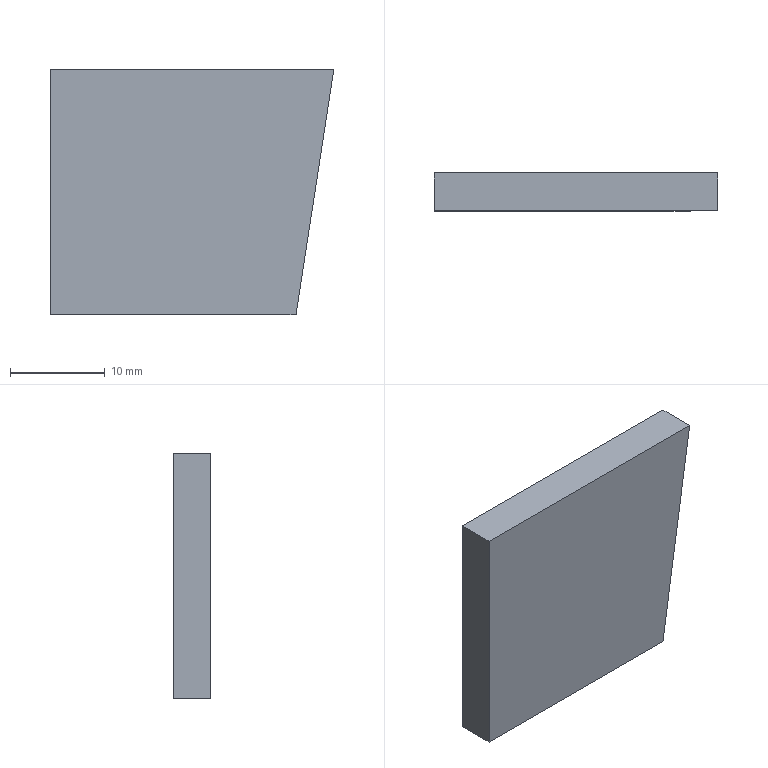Part | SolidWorks | features Extrusion 1 | 1 solid | 6 faces | box 30 x 4 x 26 mm | volume 2912 mm3 | plane 6
STEP:
#1=CARTESIAN_POINT('',(0.,0.,0.));
#2=VERTEX_POINT('',#1);
#3=CARTESIAN_POINT('',(30.,0.,0.));
#4=VERTEX_POINT('',#3);
#5=CARTESIAN_POINT('',(30.,0.,0.));
#6=DIRECTION('',(1.,0.,0.));
#7=VECTOR('',#6,1000.);
#8=LINE('',#5,#7);
#9=EDGE_CURVE('',#2,#4,#8,.T.);
#10=ORIENTED_EDGE('',*,*,#9,.T.);
#11=CARTESIAN_POINT('',(30.,4.,0.));
#12=VERTEX_POINT('',#11);
#13=CARTESIAN_POINT('',(30.,4.,0.));
#14=DIRECTION('',(0.,-1.,0.));
#15=VECTOR('',#14,1000.);
#16=LINE('',#13,#15);
#17=EDGE_CURVE('',#12,#4,#16,.T.);
#18=ORIENTED_EDGE('',*,*,#17,.F.);
#19=CARTESIAN_POINT('',(0.,4.,0.));
#20=VERTEX_POINT('',#19);
#21=CARTESIAN_POINT('',(30.,4.,0.));
#22=DIRECTION('',(1.,0.,0.));
#23=VECTOR('',#22,1000.);
#24=LINE('',#21,#23);
#25=EDGE_CURVE('',#20,#12,#24,.T.);
#26=ORIENTED_EDGE('',*,*,#25,.F.);
#27=CARTESIAN_POINT('',(0.,4.,0.));
#28=DIRECTION('',(0.,-1.,0.));
#29=VECTOR('',#28,1000.);
#30=LINE('',#27,#29);
#31=EDGE_CURVE('',#20,#2,#30,.T.);
#32=ORIENTED_EDGE('',*,*,#31,.T.);
#33=EDGE_LOOP('',(#10,#18,#26,#32));
#34=FACE_OUTER_BOUND('',#33,.T.);
#35=CARTESIAN_POINT('',(30.,4.,0.));
#36=DIRECTION('',(0.,0.,-1.));
#37=DIRECTION('',(-1.,0.,0.));
#38=AXIS2_PLACEMENT_3D('',#35,#36,#37);
#39=PLANE('',#38);
#40=ADVANCED_FACE('',(#34),#39,.F.);
#41=CARTESIAN_POINT('',(26.,0.,-26.));
#42=VERTEX_POINT('',#41);
#43=CARTESIAN_POINT('',(26.,0.,-26.));
#44=DIRECTION('',(-0.1521,0.,-0.9884));
#45=VECTOR('',#44,1000.);
#46=LINE('',#43,#45);
#47=EDGE_CURVE('',#4,#42,#46,.T.);
#48=ORIENTED_EDGE('',*,*,#47,.T.);
#49=CARTESIAN_POINT('',(26.,4.,-26.));
#50=VERTEX_POINT('',#49);
#51=CARTESIAN_POINT('',(26.,4.,-26.));
#52=DIRECTION('',(0.,-1.,0.));
#53=VECTOR('',#52,1000.);
#54=LINE('',#51,#53);
#55=EDGE_CURVE('',#50,#42,#54,.T.);
#56=ORIENTED_EDGE('',*,*,#55,.F.);
#57=CARTESIAN_POINT('',(26.,4.,-26.));
#58=DIRECTION('',(-0.1521,0.,-0.9884));
#59=VECTOR('',#58,1000.);
#60=LINE('',#57,#59);
#61=EDGE_CURVE('',#12,#50,#60,.T.);
#62=ORIENTED_EDGE('',*,*,#61,.F.);
#63=ORIENTED_EDGE('',*,*,#17,.T.);
#64=EDGE_LOOP('',(#48,#56,#62,#63));
#65=FACE_OUTER_BOUND('',#64,.T.);
#66=CARTESIAN_POINT('',(26.,4.,-26.));
#67=DIRECTION('',(-0.9884,0.,0.1521));
#68=DIRECTION('',(0.1521,0.,0.9884));
#69=AXIS2_PLACEMENT_3D('',#66,#67,#68);
#70=PLANE('',#69);
#71=ADVANCED_FACE('',(#65),#70,.F.);
#72=CARTESIAN_POINT('',(0.,0.,-26.));
#73=VERTEX_POINT('',#72);
#74=CARTESIAN_POINT('',(0.,0.,-26.));
#75=DIRECTION('',(-1.,0.,0.));
#76=VECTOR('',#75,1000.);
#77=LINE('',#74,#76);
#78=EDGE_CURVE('',#42,#73,#77,.T.);
#79=ORIENTED_EDGE('',*,*,#78,.T.);
#80=CARTESIAN_POINT('',(0.,4.,-26.));
#81=VERTEX_POINT('',#80);
#82=CARTESIAN_POINT('',(0.,4.,-26.));
#83=DIRECTION('',(0.,-1.,0.));
#84=VECTOR('',#83,1000.);
#85=LINE('',#82,#84);
#86=EDGE_CURVE('',#81,#73,#85,.T.);
#87=ORIENTED_EDGE('',*,*,#86,.F.);
#88=CARTESIAN_POINT('',(0.,4.,-26.));
#89=DIRECTION('',(-1.,0.,0.));
#90=VECTOR('',#89,1000.);
#91=LINE('',#88,#90);
#92=EDGE_CURVE('',#50,#81,#91,.T.);
#93=ORIENTED_EDGE('',*,*,#92,.F.);
#94=ORIENTED_EDGE('',*,*,#55,.T.);
#95=EDGE_LOOP('',(#79,#87,#93,#94));
#96=FACE_OUTER_BOUND('',#95,.T.);
#97=CARTESIAN_POINT('',(0.,4.,-26.));
#98=DIRECTION('',(0.,0.,1.));
#99=DIRECTION('',(1.,0.,0.));
#100=AXIS2_PLACEMENT_3D('',#97,#98,#99);
#101=PLANE('',#100);
#102=ADVANCED_FACE('',(#96),#101,.F.);
#103=CARTESIAN_POINT('',(0.,0.,0.));
#104=DIRECTION('',(0.,0.,1.));
#105=VECTOR('',#104,1000.);
#106=LINE('',#103,#105);
#107=EDGE_CURVE('',#73,#2,#106,.T.);
#108=ORIENTED_EDGE('',*,*,#107,.T.);
#109=ORIENTED_EDGE('',*,*,#31,.F.);
#110=CARTESIAN_POINT('',(0.,4.,0.));
#111=DIRECTION('',(0.,0.,1.));
#112=VECTOR('',#111,1000.);
#113=LINE('',#110,#112);
#114=EDGE_CURVE('',#81,#20,#113,.T.);
#115=ORIENTED_EDGE('',*,*,#114,.F.);
#116=ORIENTED_EDGE('',*,*,#86,.T.);
#117=EDGE_LOOP('',(#108,#109,#115,#116));
#118=FACE_OUTER_BOUND('',#117,.T.);
#119=CARTESIAN_POINT('',(0.,4.,0.));
#120=DIRECTION('',(1.,0.,0.));
#121=DIRECTION('',(0.,0.,-1.));
#122=AXIS2_PLACEMENT_3D('',#119,#120,#121);
#123=PLANE('',#122);
#124=ADVANCED_FACE('',(#118),#123,.F.);
#125=ORIENTED_EDGE('',*,*,#25,.T.);
#126=ORIENTED_EDGE('',*,*,#61,.T.);
#127=ORIENTED_EDGE('',*,*,#92,.T.);
#128=ORIENTED_EDGE('',*,*,#114,.T.);
#129=EDGE_LOOP('',(#125,#126,#127,#128));
#130=FACE_OUTER_BOUND('',#129,.T.);
#131=CARTESIAN_POINT('',(0.,4.,0.));
#132=DIRECTION('',(0.,-1.,0.));
#133=DIRECTION('',(0.,0.,-1.));
#134=AXIS2_PLACEMENT_3D('',#131,#132,#133);
#135=PLANE('',#134);
#136=ADVANCED_FACE('',(#130),#135,.F.);
#137=ORIENTED_EDGE('',*,*,#9,.F.);
#138=ORIENTED_EDGE('',*,*,#107,.F.);
#139=ORIENTED_EDGE('',*,*,#78,.F.);
#140=ORIENTED_EDGE('',*,*,#47,.F.);
#141=EDGE_LOOP('',(#137,#138,#139,#140));
#142=FACE_OUTER_BOUND('',#141,.T.);
#143=CARTESIAN_POINT('',(0.,0.,0.));
#144=DIRECTION('',(0.,-1.,0.));
#145=DIRECTION('',(0.,0.,-1.));
#146=AXIS2_PLACEMENT_3D('',#143,#144,#145);
#147=PLANE('',#146);
#148=ADVANCED_FACE('',(#142),#147,.T.);
#149=CLOSED_SHELL('',(#40,#71,#102,#124,#136,#148));
#150=MANIFOLD_SOLID_BREP('',#149);
#151=CARTESIAN_POINT('',(0.,0.,0.));
#152=DIRECTION('',(0.,0.,1.));
#153=DIRECTION('',(1.,0.,0.));
#154=AXIS2_PLACEMENT_3D('',#151,#152,#153);
#155=(LENGTH_UNIT()NAMED_UNIT(*)SI_UNIT(.MILLI.,.METRE.));
#156=UNCERTAINTY_MEASURE_WITH_UNIT(LENGTH_MEASURE(0.00001),#155,'','');
#157=(NAMED_UNIT(*)PLANE_ANGLE_UNIT()SI_UNIT($,.RADIAN.));
#158=(NAMED_UNIT(*)SI_UNIT($,.STERADIAN.)SOLID_ANGLE_UNIT());
#159=(GEOMETRIC_REPRESENTATION_CONTEXT(3)GLOBAL_UNCERTAINTY_ASSIGNED_CONTEXT((#156))GLOBAL_UNIT_ASSIGNED_CONTEXT((#155,#157,#158))REPRESENTATION_CONTEXT('',''));
#160=ADVANCED_BREP_SHAPE_REPRESENTATION('',(#150,#154),#159);